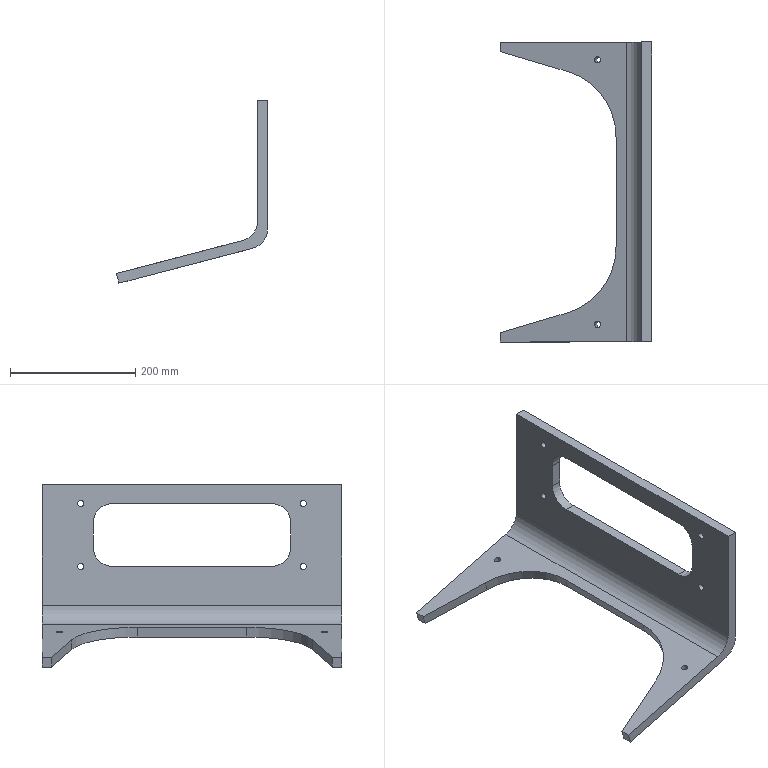Part | SolidWorks | features HoleWzd 2, ICE 2, Extrusion 1 | 1 solid | 48 faces | box 241.053 x 478 x 290.926 mm | volume 1872027 mm3 | cylinder 20 | plane 16 | cone 12 | commonest cylinder face diameters 10.2 x12 60.6 x4 64 x2 218.4 x2
STEP:
#1=CARTESIAN_POINT('',(2428.148,450.,-1751.717));
#2=VERTEX_POINT('',#1);
#3=CARTESIAN_POINT('',(2418.279,450.,-1754.295));
#4=VERTEX_POINT('',#3);
#5=CARTESIAN_POINT('',(2423.214,450.,-1753.006));
#6=DIRECTION('',(0.2527,0.,-0.9675));
#7=DIRECTION('',(-0.9675,0.,-0.2527));
#8=AXIS2_PLACEMENT_3D('',#5,#6,#7);
#9=CIRCLE('',#8,5.1);
#10=EDGE_CURVE('',#2,#4,#9,.T.);
#11=ORIENTED_EDGE('',*,*,#10,.F.);
#12=CARTESIAN_POINT('',(2429.277,450.,-1752.378));
#13=VERTEX_POINT('',#12);
#14=CARTESIAN_POINT('',(2429.277,450.,-1752.378));
#15=DIRECTION('',(0.8629,0.,-0.5054));
#16=VECTOR('',#15,1000.);
#17=LINE('',#14,#16);
#18=EDGE_CURVE('',#2,#13,#17,.T.);
#19=ORIENTED_EDGE('',*,*,#18,.T.);
#20=CARTESIAN_POINT('',(2417.618,450.,-1755.424));
#21=VERTEX_POINT('',#20);
#22=CARTESIAN_POINT('',(2423.447,450.,-1753.901));
#23=DIRECTION('',(0.2527,0.,-0.9675));
#24=DIRECTION('',(-0.9675,0.,-0.2527));
#25=AXIS2_PLACEMENT_3D('',#22,#23,#24);
#26=CIRCLE('',#25,6.025);
#27=EDGE_CURVE('',#13,#21,#26,.T.);
#28=ORIENTED_EDGE('',*,*,#27,.T.);
#29=CARTESIAN_POINT('',(2417.618,450.,-1755.424));
#30=DIRECTION('',(-0.5054,0.,-0.8629));
#31=VECTOR('',#30,1000.);
#32=LINE('',#29,#31);
#33=EDGE_CURVE('',#4,#21,#32,.T.);
#34=ORIENTED_EDGE('',*,*,#33,.F.);
#35=EDGE_LOOP('',(#11,#19,#28,#34));
#36=FACE_OUTER_BOUND('',#35,.T.);
#37=CARTESIAN_POINT('',(2423.447,450.,-1753.901));
#38=DIRECTION('',(0.2527,0.,-0.9675));
#39=DIRECTION('',(-0.9675,0.,-0.2527));
#40=AXIS2_PLACEMENT_3D('',#37,#38,#39);
#41=CONICAL_SURFACE('',#40,6.025,0.7854);
#42=ADVANCED_FACE('',(#36),#41,.F.);
#43=CARTESIAN_POINT('',(2424.338,450.,-1737.131));
#44=VERTEX_POINT('',#43);
#45=CARTESIAN_POINT('',(2414.469,450.,-1739.709));
#46=VERTEX_POINT('',#45);
#47=CARTESIAN_POINT('',(2419.403,450.,-1738.42));
#48=DIRECTION('',(0.2527,0.,-0.9675));
#49=DIRECTION('',(-0.9675,0.,-0.2527));
#50=AXIS2_PLACEMENT_3D('',#47,#48,#49);
#51=CIRCLE('',#50,5.1);
#52=EDGE_CURVE('',#44,#46,#51,.T.);
#53=ORIENTED_EDGE('',*,*,#52,.F.);
#54=CARTESIAN_POINT('',(2428.382,450.,-1752.612));
#55=DIRECTION('',(0.2527,0.,-0.9675));
#56=VECTOR('',#55,1000.);
#57=LINE('',#54,#56);
#58=EDGE_CURVE('',#44,#2,#57,.T.);
#59=ORIENTED_EDGE('',*,*,#58,.T.);
#60=ORIENTED_EDGE('',*,*,#10,.T.);
#61=CARTESIAN_POINT('',(2418.513,450.,-1755.19));
#62=DIRECTION('',(0.2527,0.,-0.9675));
#63=VECTOR('',#62,1000.);
#64=LINE('',#61,#63);
#65=EDGE_CURVE('',#46,#4,#64,.T.);
#66=ORIENTED_EDGE('',*,*,#65,.F.);
#67=EDGE_LOOP('',(#53,#59,#60,#66));
#68=FACE_OUTER_BOUND('',#67,.T.);
#69=CARTESIAN_POINT('',(2423.447,450.,-1753.901));
#70=DIRECTION('',(0.2527,0.,-0.9675));
#71=DIRECTION('',(-0.9675,0.,-0.2527));
#72=AXIS2_PLACEMENT_3D('',#69,#70,#71);
#73=CYLINDRICAL_SURFACE('',#72,5.1);
#74=ADVANCED_FACE('',(#68),#73,.F.);
#75=CARTESIAN_POINT('',(2428.148,28.,-1751.717));
#76=VERTEX_POINT('',#75);
#77=CARTESIAN_POINT('',(2418.279,28.,-1754.295));
#78=VERTEX_POINT('',#77);
#79=CARTESIAN_POINT('',(2423.214,28.,-1753.006));
#80=DIRECTION('',(0.2527,0.,-0.9675));
#81=DIRECTION('',(-0.9675,0.,-0.2527));
#82=AXIS2_PLACEMENT_3D('',#79,#80,#81);
#83=CIRCLE('',#82,5.1);
#84=EDGE_CURVE('',#76,#78,#83,.T.);
#85=ORIENTED_EDGE('',*,*,#84,.F.);
#86=CARTESIAN_POINT('',(2429.277,28.,-1752.378));
#87=VERTEX_POINT('',#86);
#88=CARTESIAN_POINT('',(2429.277,28.,-1752.378));
#89=DIRECTION('',(0.8629,0.,-0.5054));
#90=VECTOR('',#89,1000.);
#91=LINE('',#88,#90);
#92=EDGE_CURVE('',#76,#87,#91,.T.);
#93=ORIENTED_EDGE('',*,*,#92,.T.);
#94=CARTESIAN_POINT('',(2417.618,28.,-1755.424));
#95=VERTEX_POINT('',#94);
#96=CARTESIAN_POINT('',(2423.447,28.,-1753.901));
#97=DIRECTION('',(0.2527,0.,-0.9675));
#98=DIRECTION('',(-0.9675,0.,-0.2527));
#99=AXIS2_PLACEMENT_3D('',#96,#97,#98);
#100=CIRCLE('',#99,6.025);
#101=EDGE_CURVE('',#87,#95,#100,.T.);
#102=ORIENTED_EDGE('',*,*,#101,.T.);
#103=CARTESIAN_POINT('',(2417.618,28.,-1755.424));
#104=DIRECTION('',(-0.5054,0.,-0.8629));
#105=VECTOR('',#104,1000.);
#106=LINE('',#103,#105);
#107=EDGE_CURVE('',#78,#95,#106,.T.);
#108=ORIENTED_EDGE('',*,*,#107,.F.);
#109=EDGE_LOOP('',(#85,#93,#102,#108));
#110=FACE_OUTER_BOUND('',#109,.T.);
#111=CARTESIAN_POINT('',(2423.447,28.,-1753.901));
#112=DIRECTION('',(0.2527,0.,-0.9675));
#113=DIRECTION('',(-0.9675,0.,-0.2527));
#114=AXIS2_PLACEMENT_3D('',#111,#112,#113);
#115=CONICAL_SURFACE('',#114,6.025,0.7854);
#116=ADVANCED_FACE('',(#110),#115,.F.);
#117=CARTESIAN_POINT('',(2424.338,28.,-1737.131));
#118=VERTEX_POINT('',#117);
#119=CARTESIAN_POINT('',(2414.469,28.,-1739.709));
#120=VERTEX_POINT('',#119);
#121=CARTESIAN_POINT('',(2419.403,28.,-1738.42));
#122=DIRECTION('',(0.2527,0.,-0.9675));
#123=DIRECTION('',(-0.9675,0.,-0.2527));
#124=AXIS2_PLACEMENT_3D('',#121,#122,#123);
#125=CIRCLE('',#124,5.1);
#126=EDGE_CURVE('',#118,#120,#125,.T.);
#127=ORIENTED_EDGE('',*,*,#126,.F.);
#128=CARTESIAN_POINT('',(2428.382,28.,-1752.612));
#129=DIRECTION('',(0.2527,0.,-0.9675));
#130=VECTOR('',#129,1000.);
#131=LINE('',#128,#130);
#132=EDGE_CURVE('',#118,#76,#131,.T.);
#133=ORIENTED_EDGE('',*,*,#132,.T.);
#134=ORIENTED_EDGE('',*,*,#84,.T.);
#135=CARTESIAN_POINT('',(2418.513,28.,-1755.19));
#136=DIRECTION('',(0.2527,0.,-0.9675));
#137=VECTOR('',#136,1000.);
#138=LINE('',#135,#137);
#139=EDGE_CURVE('',#120,#78,#138,.T.);
#140=ORIENTED_EDGE('',*,*,#139,.F.);
#141=EDGE_LOOP('',(#127,#133,#134,#140));
#142=FACE_OUTER_BOUND('',#141,.T.);
#143=CARTESIAN_POINT('',(2423.447,28.,-1753.901));
#144=DIRECTION('',(0.2527,0.,-0.9675));
#145=DIRECTION('',(-0.9675,0.,-0.2527));
#146=AXIS2_PLACEMENT_3D('',#143,#144,#145);
#147=CYLINDRICAL_SURFACE('',#146,5.1);
#148=ADVANCED_FACE('',(#142),#147,.F.);
#149=CARTESIAN_POINT('',(2504.822,416.55,-1628.488));
#150=VERTEX_POINT('',#149);
#151=CARTESIAN_POINT('',(2504.822,416.55,-1638.688));
#152=VERTEX_POINT('',#151);
#153=CARTESIAN_POINT('',(2504.822,416.55,-1633.588));
#154=DIRECTION('',(1.,0.,0.));
#155=DIRECTION('',(0.,0.,-1.));
#156=AXIS2_PLACEMENT_3D('',#153,#154,#155);
#157=CIRCLE('',#156,5.1);
#158=EDGE_CURVE('',#150,#152,#157,.T.);
#159=ORIENTED_EDGE('',*,*,#158,.F.);
#160=CARTESIAN_POINT('',(2505.747,416.55,-1627.563));
#161=VERTEX_POINT('',#160);
#162=CARTESIAN_POINT('',(2505.747,416.55,-1627.563));
#163=DIRECTION('',(0.7071,0.,0.7071));
#164=VECTOR('',#163,1000.);
#165=LINE('',#162,#164);
#166=EDGE_CURVE('',#150,#161,#165,.T.);
#167=ORIENTED_EDGE('',*,*,#166,.T.);
#168=CARTESIAN_POINT('',(2505.747,416.55,-1639.613));
#169=VERTEX_POINT('',#168);
#170=CARTESIAN_POINT('',(2505.747,416.55,-1633.588));
#171=DIRECTION('',(1.,0.,0.));
#172=DIRECTION('',(0.,0.,-1.));
#173=AXIS2_PLACEMENT_3D('',#170,#171,#172);
#174=CIRCLE('',#173,6.025);
#175=EDGE_CURVE('',#161,#169,#174,.T.);
#176=ORIENTED_EDGE('',*,*,#175,.T.);
#177=CARTESIAN_POINT('',(2505.747,416.55,-1639.613));
#178=DIRECTION('',(0.7071,0.,-0.7071));
#179=VECTOR('',#178,1000.);
#180=LINE('',#177,#179);
#181=EDGE_CURVE('',#152,#169,#180,.T.);
#182=ORIENTED_EDGE('',*,*,#181,.F.);
#183=EDGE_LOOP('',(#159,#167,#176,#182));
#184=FACE_OUTER_BOUND('',#183,.T.);
#185=CARTESIAN_POINT('',(2505.747,416.55,-1633.588));
#186=DIRECTION('',(1.,0.,0.));
#187=DIRECTION('',(0.,0.,-1.));
#188=AXIS2_PLACEMENT_3D('',#185,#186,#187);
#189=CONICAL_SURFACE('',#188,6.025,0.7854);
#190=ADVANCED_FACE('',(#184),#189,.F.);
#191=CARTESIAN_POINT('',(2489.747,416.55,-1628.488));
#192=VERTEX_POINT('',#191);
#193=CARTESIAN_POINT('',(2489.747,416.55,-1638.688));
#194=VERTEX_POINT('',#193);
#195=CARTESIAN_POINT('',(2489.747,416.55,-1633.588));
#196=DIRECTION('',(1.,0.,0.));
#197=DIRECTION('',(0.,0.,-1.));
#198=AXIS2_PLACEMENT_3D('',#195,#196,#197);
#199=CIRCLE('',#198,5.1);
#200=EDGE_CURVE('',#192,#194,#199,.T.);
#201=ORIENTED_EDGE('',*,*,#200,.F.);
#202=CARTESIAN_POINT('',(2505.747,416.55,-1628.488));
#203=DIRECTION('',(1.,0.,0.));
#204=VECTOR('',#203,1000.);
#205=LINE('',#202,#204);
#206=EDGE_CURVE('',#192,#150,#205,.T.);
#207=ORIENTED_EDGE('',*,*,#206,.T.);
#208=ORIENTED_EDGE('',*,*,#158,.T.);
#209=CARTESIAN_POINT('',(2505.747,416.55,-1638.688));
#210=DIRECTION('',(1.,0.,0.));
#211=VECTOR('',#210,1000.);
#212=LINE('',#209,#211);
#213=EDGE_CURVE('',#194,#152,#212,.T.);
#214=ORIENTED_EDGE('',*,*,#213,.F.);
#215=EDGE_LOOP('',(#201,#207,#208,#214));
#216=FACE_OUTER_BOUND('',#215,.T.);
#217=CARTESIAN_POINT('',(2505.747,416.55,-1633.588));
#218=DIRECTION('',(1.,0.,0.));
#219=DIRECTION('',(0.,0.,-1.));
#220=AXIS2_PLACEMENT_3D('',#217,#218,#219);
#221=CYLINDRICAL_SURFACE('',#220,5.1);
#222=ADVANCED_FACE('',(#216),#221,.F.);
#223=CARTESIAN_POINT('',(2504.822,61.45,-1528.288));
#224=VERTEX_POINT('',#223);
#225=CARTESIAN_POINT('',(2504.822,61.45,-1538.488));
#226=VERTEX_POINT('',#225);
#227=CARTESIAN_POINT('',(2504.822,61.45,-1533.388));
#228=DIRECTION('',(1.,0.,0.));
#229=DIRECTION('',(0.,0.,-1.));
#230=AXIS2_PLACEMENT_3D('',#227,#228,#229);
#231=CIRCLE('',#230,5.1);
#232=EDGE_CURVE('',#224,#226,#231,.T.);
#233=ORIENTED_EDGE('',*,*,#232,.F.);
#234=CARTESIAN_POINT('',(2505.747,61.45,-1527.363));
#235=VERTEX_POINT('',#234);
#236=CARTESIAN_POINT('',(2505.747,61.45,-1527.363));
#237=DIRECTION('',(0.7071,0.,0.7071));
#238=VECTOR('',#237,1000.);
#239=LINE('',#236,#238);
#240=EDGE_CURVE('',#224,#235,#239,.T.);
#241=ORIENTED_EDGE('',*,*,#240,.T.);
#242=CARTESIAN_POINT('',(2505.747,61.45,-1539.413));
#243=VERTEX_POINT('',#242);
#244=CARTESIAN_POINT('',(2505.747,61.45,-1533.388));
#245=DIRECTION('',(1.,0.,0.));
#246=DIRECTION('',(0.,0.,-1.));
#247=AXIS2_PLACEMENT_3D('',#244,#245,#246);
#248=CIRCLE('',#247,6.025);
#249=EDGE_CURVE('',#235,#243,#248,.T.);
#250=ORIENTED_EDGE('',*,*,#249,.T.);
#251=CARTESIAN_POINT('',(2505.747,61.45,-1539.413));
#252=DIRECTION('',(0.7071,0.,-0.7071));
#253=VECTOR('',#252,1000.);
#254=LINE('',#251,#253);
#255=EDGE_CURVE('',#226,#243,#254,.T.);
#256=ORIENTED_EDGE('',*,*,#255,.F.);
#257=EDGE_LOOP('',(#233,#241,#250,#256));
#258=FACE_OUTER_BOUND('',#257,.T.);
#259=CARTESIAN_POINT('',(2505.747,61.45,-1533.388));
#260=DIRECTION('',(1.,0.,0.));
#261=DIRECTION('',(0.,0.,-1.));
#262=AXIS2_PLACEMENT_3D('',#259,#260,#261);
#263=CONICAL_SURFACE('',#262,6.025,0.7854);
#264=ADVANCED_FACE('',(#258),#263,.F.);
#265=CARTESIAN_POINT('',(2489.747,61.45,-1528.288));
#266=VERTEX_POINT('',#265);
#267=CARTESIAN_POINT('',(2489.747,61.45,-1538.488));
#268=VERTEX_POINT('',#267);
#269=CARTESIAN_POINT('',(2489.747,61.45,-1533.388));
#270=DIRECTION('',(1.,0.,0.));
#271=DIRECTION('',(0.,0.,-1.));
#272=AXIS2_PLACEMENT_3D('',#269,#270,#271);
#273=CIRCLE('',#272,5.1);
#274=EDGE_CURVE('',#266,#268,#273,.T.);
#275=ORIENTED_EDGE('',*,*,#274,.F.);
#276=CARTESIAN_POINT('',(2505.747,61.45,-1528.288));
#277=DIRECTION('',(1.,0.,0.));
#278=VECTOR('',#277,1000.);
#279=LINE('',#276,#278);
#280=EDGE_CURVE('',#266,#224,#279,.T.);
#281=ORIENTED_EDGE('',*,*,#280,.T.);
#282=ORIENTED_EDGE('',*,*,#232,.T.);
#283=CARTESIAN_POINT('',(2505.747,61.45,-1538.488));
#284=DIRECTION('',(1.,0.,0.));
#285=VECTOR('',#284,1000.);
#286=LINE('',#283,#285);
#287=EDGE_CURVE('',#268,#226,#286,.T.);
#288=ORIENTED_EDGE('',*,*,#287,.F.);
#289=EDGE_LOOP('',(#275,#281,#282,#288));
#290=FACE_OUTER_BOUND('',#289,.T.);
#291=CARTESIAN_POINT('',(2505.747,61.45,-1533.388));
#292=DIRECTION('',(1.,0.,0.));
#293=DIRECTION('',(0.,0.,-1.));
#294=AXIS2_PLACEMENT_3D('',#291,#292,#293);
#295=CYLINDRICAL_SURFACE('',#294,5.1);
#296=ADVANCED_FACE('',(#290),#295,.F.);
#297=CARTESIAN_POINT('',(2504.822,416.55,-1528.288));
#298=VERTEX_POINT('',#297);
#299=CARTESIAN_POINT('',(2504.822,416.55,-1538.488));
#300=VERTEX_POINT('',#299);
#301=CARTESIAN_POINT('',(2504.822,416.55,-1533.388));
#302=DIRECTION('',(1.,0.,0.));
#303=DIRECTION('',(0.,0.,-1.));
#304=AXIS2_PLACEMENT_3D('',#301,#302,#303);
#305=CIRCLE('',#304,5.1);
#306=EDGE_CURVE('',#298,#300,#305,.T.);
#307=ORIENTED_EDGE('',*,*,#306,.F.);
#308=CARTESIAN_POINT('',(2505.747,416.55,-1527.363));
#309=VERTEX_POINT('',#308);
#310=CARTESIAN_POINT('',(2505.747,416.55,-1527.363));
#311=DIRECTION('',(0.7071,0.,0.7071));
#312=VECTOR('',#311,1000.);
#313=LINE('',#310,#312);
#314=EDGE_CURVE('',#298,#309,#313,.T.);
#315=ORIENTED_EDGE('',*,*,#314,.T.);
#316=CARTESIAN_POINT('',(2505.747,416.55,-1539.413));
#317=VERTEX_POINT('',#316);
#318=CARTESIAN_POINT('',(2505.747,416.55,-1533.388));
#319=DIRECTION('',(1.,0.,0.));
#320=DIRECTION('',(0.,0.,-1.));
#321=AXIS2_PLACEMENT_3D('',#318,#319,#320);
#322=CIRCLE('',#321,6.025);
#323=EDGE_CURVE('',#309,#317,#322,.T.);
#324=ORIENTED_EDGE('',*,*,#323,.T.);
#325=CARTESIAN_POINT('',(2505.747,416.55,-1539.413));
#326=DIRECTION('',(0.7071,0.,-0.7071));
#327=VECTOR('',#326,1000.);
#328=LINE('',#325,#327);
#329=EDGE_CURVE('',#300,#317,#328,.T.);
#330=ORIENTED_EDGE('',*,*,#329,.F.);
#331=EDGE_LOOP('',(#307,#315,#324,#330));
#332=FACE_OUTER_BOUND('',#331,.T.);
#333=CARTESIAN_POINT('',(2505.747,416.55,-1533.388));
#334=DIRECTION('',(1.,0.,0.));
#335=DIRECTION('',(0.,0.,-1.));
#336=AXIS2_PLACEMENT_3D('',#333,#334,#335);
#337=CONICAL_SURFACE('',#336,6.025,0.7854);
#338=ADVANCED_FACE('',(#332),#337,.F.);
#339=CARTESIAN_POINT('',(2489.747,416.55,-1528.288));
#340=VERTEX_POINT('',#339);
#341=CARTESIAN_POINT('',(2489.747,416.55,-1538.488));
#342=VERTEX_POINT('',#341);
#343=CARTESIAN_POINT('',(2489.747,416.55,-1533.388));
#344=DIRECTION('',(1.,0.,0.));
#345=DIRECTION('',(0.,0.,-1.));
#346=AXIS2_PLACEMENT_3D('',#343,#344,#345);
#347=CIRCLE('',#346,5.1);
#348=EDGE_CURVE('',#340,#342,#347,.T.);
#349=ORIENTED_EDGE('',*,*,#348,.F.);
#350=CARTESIAN_POINT('',(2505.747,416.55,-1528.288));
#351=DIRECTION('',(1.,0.,0.));
#352=VECTOR('',#351,1000.);
#353=LINE('',#350,#352);
#354=EDGE_CURVE('',#340,#298,#353,.T.);
#355=ORIENTED_EDGE('',*,*,#354,.T.);
#356=ORIENTED_EDGE('',*,*,#306,.T.);
#357=CARTESIAN_POINT('',(2505.747,416.55,-1538.488));
#358=DIRECTION('',(1.,0.,0.));
#359=VECTOR('',#358,1000.);
#360=LINE('',#357,#359);
#361=EDGE_CURVE('',#342,#300,#360,.T.);
#362=ORIENTED_EDGE('',*,*,#361,.F.);
#363=EDGE_LOOP('',(#349,#355,#356,#362));
#364=FACE_OUTER_BOUND('',#363,.T.);
#365=CARTESIAN_POINT('',(2505.747,416.55,-1533.388));
#366=DIRECTION('',(1.,0.,0.));
#367=DIRECTION('',(0.,0.,-1.));
#368=AXIS2_PLACEMENT_3D('',#365,#366,#367);
#369=CYLINDRICAL_SURFACE('',#368,5.1);
#370=ADVANCED_FACE('',(#364),#369,.F.);
#371=CARTESIAN_POINT('',(2504.822,61.45,-1628.488));
#372=VERTEX_POINT('',#371);
#373=CARTESIAN_POINT('',(2504.822,61.45,-1638.688));
#374=VERTEX_POINT('',#373);
#375=CARTESIAN_POINT('',(2504.822,61.45,-1633.588));
#376=DIRECTION('',(1.,0.,0.));
#377=DIRECTION('',(0.,0.,-1.));
#378=AXIS2_PLACEMENT_3D('',#375,#376,#377);
#379=CIRCLE('',#378,5.1);
#380=EDGE_CURVE('',#372,#374,#379,.T.);
#381=ORIENTED_EDGE('',*,*,#380,.F.);
#382=CARTESIAN_POINT('',(2505.747,61.45,-1627.563));
#383=VERTEX_POINT('',#382);
#384=CARTESIAN_POINT('',(2505.747,61.45,-1627.563));
#385=DIRECTION('',(0.7071,0.,0.7071));
#386=VECTOR('',#385,1000.);
#387=LINE('',#384,#386);
#388=EDGE_CURVE('',#372,#383,#387,.T.);
#389=ORIENTED_EDGE('',*,*,#388,.T.);
#390=CARTESIAN_POINT('',(2505.747,61.45,-1639.613));
#391=VERTEX_POINT('',#390);
#392=CARTESIAN_POINT('',(2505.747,61.45,-1633.588));
#393=DIRECTION('',(1.,0.,0.));
#394=DIRECTION('',(0.,0.,-1.));
#395=AXIS2_PLACEMENT_3D('',#392,#393,#394);
#396=CIRCLE('',#395,6.025);
#397=EDGE_CURVE('',#383,#391,#396,.T.);
#398=ORIENTED_EDGE('',*,*,#397,.T.);
#399=CARTESIAN_POINT('',(2505.747,61.45,-1639.613));
#400=DIRECTION('',(0.7071,0.,-0.7071));
#401=VECTOR('',#400,1000.);
#402=LINE('',#399,#401);
#403=EDGE_CURVE('',#374,#391,#402,.T.);
#404=ORIENTED_EDGE('',*,*,#403,.F.);
#405=EDGE_LOOP('',(#381,#389,#398,#404));
#406=FACE_OUTER_BOUND('',#405,.T.);
#407=CARTESIAN_POINT('',(2505.747,61.45,-1633.588));
#408=DIRECTION('',(1.,0.,0.));
#409=DIRECTION('',(0.,0.,-1.));
#410=AXIS2_PLACEMENT_3D('',#407,#408,#409);
#411=CONICAL_SURFACE('',#410,6.025,0.7854);
#412=ADVANCED_FACE('',(#406),#411,.F.);
#413=CARTESIAN_POINT('',(2489.747,61.45,-1628.488));
#414=VERTEX_POINT('',#413);
#415=CARTESIAN_POINT('',(2489.747,61.45,-1638.688));
#416=VERTEX_POINT('',#415);
#417=CARTESIAN_POINT('',(2489.747,61.45,-1633.588));
#418=DIRECTION('',(1.,0.,0.));
#419=DIRECTION('',(0.,0.,-1.));
#420=AXIS2_PLACEMENT_3D('',#417,#418,#419);
#421=CIRCLE('',#420,5.1);
#422=EDGE_CURVE('',#414,#416,#421,.T.);
#423=ORIENTED_EDGE('',*,*,#422,.F.);
#424=CARTESIAN_POINT('',(2505.747,61.45,-1628.488));
#425=DIRECTION('',(1.,0.,0.));
#426=VECTOR('',#425,1000.);
#427=LINE('',#424,#426);
#428=EDGE_CURVE('',#414,#372,#427,.T.);
#429=ORIENTED_EDGE('',*,*,#428,.T.);
#430=ORIENTED_EDGE('',*,*,#380,.T.);
#431=CARTESIAN_POINT('',(2505.747,61.45,-1638.688));
#432=DIRECTION('',(1.,0.,0.));
#433=VECTOR('',#432,1000.);
#434=LINE('',#431,#433);
#435=EDGE_CURVE('',#416,#374,#434,.T.);
#436=ORIENTED_EDGE('',*,*,#435,.F.);
#437=EDGE_LOOP('',(#423,#429,#430,#436));
#438=FACE_OUTER_BOUND('',#437,.T.);
#439=CARTESIAN_POINT('',(2505.747,61.45,-1633.588));
#440=DIRECTION('',(1.,0.,0.));
#441=DIRECTION('',(0.,0.,-1.));
#442=AXIS2_PLACEMENT_3D('',#439,#440,#441);
#443=CYLINDRICAL_SURFACE('',#442,5.1);
#444=ADVANCED_FACE('',(#438),#443,.F.);
#445=CARTESIAN_POINT('',(2268.739,478.,-1794.315));
#446=VERTEX_POINT('',#445);
#447=CARTESIAN_POINT('',(2268.739,463.,-1794.315));
#448=VERTEX_POINT('',#447);
#449=CARTESIAN_POINT('',(2268.739,478.,-1794.315));
#450=DIRECTION('',(0.,-1.,0.));
#451=VECTOR('',#450,1000.);
#452=LINE('',#449,#451);
#453=EDGE_CURVE('',#446,#448,#452,.T.);
#454=ORIENTED_EDGE('',*,*,#453,.T.);
#455=CARTESIAN_POINT('',(2264.695,463.,-1778.834));
#456=VERTEX_POINT('',#455);
#457=CARTESIAN_POINT('',(2147.927,463.,-1331.834));
#458=DIRECTION('',(0.2527,0.,-0.9675));
#459=VECTOR('',#458,1000.);
#460=LINE('',#457,#459);
#461=EDGE_CURVE('',#456,#448,#460,.T.);
#462=ORIENTED_EDGE('',*,*,#461,.F.);
#463=CARTESIAN_POINT('',(2264.695,478.,-1778.834));
#464=VERTEX_POINT('',#463);
#465=CARTESIAN_POINT('',(2264.695,478.,-1778.834));
#466=DIRECTION('',(0.,-1.,0.));
#467=VECTOR('',#466,1000.);
#468=LINE('',#465,#467);
#469=EDGE_CURVE('',#464,#456,#468,.T.);
#470=ORIENTED_EDGE('',*,*,#469,.F.);
#471=CARTESIAN_POINT('',(2268.739,478.,-1794.315));
#472=DIRECTION('',(-0.2527,0.,0.9675));
#473=VECTOR('',#472,1000.);
#474=LINE('',#471,#473);
#475=EDGE_CURVE('',#446,#464,#474,.T.);
#476=ORIENTED_EDGE('',*,*,#475,.F.);
#477=EDGE_LOOP('',(#454,#462,#470,#476));
#478=FACE_OUTER_BOUND('',#477,.T.);
#479=CARTESIAN_POINT('',(2268.739,478.,-1794.315));
#480=DIRECTION('',(0.9675,0.,0.2527));
#481=DIRECTION('',(0.2527,0.,-0.9675));
#482=AXIS2_PLACEMENT_3D('',#479,#480,#481);
#483=PLANE('',#482);
#484=ADVANCED_FACE('',(#478),#483,.F.);
#485=CARTESIAN_POINT('',(2489.747,416.55,-1633.588));
#486=DIRECTION('',(1.,0.,0.));
#487=DIRECTION('',(0.,0.,-1.));
#488=AXIS2_PLACEMENT_3D('',#485,#486,#487);
#489=CIRCLE('',#488,5.1);
#490=EDGE_CURVE('',#194,#192,#489,.T.);
#491=ORIENTED_EDGE('',*,*,#490,.T.);
#492=ORIENTED_EDGE('',*,*,#200,.T.);
#493=EDGE_LOOP('',(#491,#492));
#494=FACE_BOUND('',#493,.T.);
#495=CARTESIAN_POINT('',(2489.747,61.45,-1533.388));
#496=DIRECTION('',(1.,0.,0.));
#497=DIRECTION('',(0.,0.,-1.));
#498=AXIS2_PLACEMENT_3D('',#495,#496,#497);
#499=CIRCLE('',#498,5.1);
#500=EDGE_CURVE('',#268,#266,#499,.T.);
#501=ORIENTED_EDGE('',*,*,#500,.T.);
#502=ORIENTED_EDGE('',*,*,#274,.T.);
#503=EDGE_LOOP('',(#501,#502));
#504=FACE_BOUND('',#503,.T.);
#505=CARTESIAN_POINT('',(2489.747,416.55,-1533.388));
#506=DIRECTION('',(1.,0.,0.));
#507=DIRECTION('',(0.,0.,-1.));
#508=AXIS2_PLACEMENT_3D('',#505,#506,#507);
#509=CIRCLE('',#508,5.1);
#510=EDGE_CURVE('',#342,#340,#509,.T.);
#511=ORIENTED_EDGE('',*,*,#510,.T.);
#512=ORIENTED_EDGE('',*,*,#348,.T.);
#513=EDGE_LOOP('',(#511,#512));
#514=FACE_BOUND('',#513,.T.);
#515=CARTESIAN_POINT('',(2489.747,61.45,-1633.588));
#516=DIRECTION('',(1.,0.,0.));
#517=DIRECTION('',(0.,0.,-1.));
#518=AXIS2_PLACEMENT_3D('',#515,#516,#517);
#519=CIRCLE('',#518,5.1);
#520=EDGE_CURVE('',#416,#414,#519,.T.);
#521=ORIENTED_EDGE('',*,*,#520,.T.);
#522=ORIENTED_EDGE('',*,*,#422,.T.);
#523=EDGE_LOOP('',(#521,#522));
#524=FACE_BOUND('',#523,.T.);
#525=CARTESIAN_POINT('',(2489.747,366.1,-1533.388));
#526=VERTEX_POINT('',#525);
#527=CARTESIAN_POINT('',(2489.747,111.9,-1533.388));
#528=VERTEX_POINT('',#527);
#529=CARTESIAN_POINT('',(2489.747,478.,-1533.388));
#530=DIRECTION('',(0.,-1.,0.));
#531=VECTOR('',#530,1000.);
#532=LINE('',#529,#531);
#533=EDGE_CURVE('',#526,#528,#532,.T.);
#534=ORIENTED_EDGE('',*,*,#533,.T.);
#535=CARTESIAN_POINT('',(2489.747,81.6,-1563.688));
#536=VERTEX_POINT('',#535);
#537=CARTESIAN_POINT('',(2489.747,111.9,-1563.688));
#538=DIRECTION('',(1.,0.,0.));
#539=DIRECTION('',(0.,0.,-1.));
#540=AXIS2_PLACEMENT_3D('',#537,#538,#539);
#541=CIRCLE('',#540,30.3);
#542=EDGE_CURVE('',#528,#536,#541,.T.);
#543=ORIENTED_EDGE('',*,*,#542,.T.);
#544=CARTESIAN_POINT('',(2489.747,81.6,-1603.288));
#545=VERTEX_POINT('',#544);
#546=CARTESIAN_POINT('',(2489.747,81.6,-1503.388));
#547=DIRECTION('',(0.,0.,-1.));
#548=VECTOR('',#547,1000.);
#549=LINE('',#546,#548);
#550=EDGE_CURVE('',#536,#545,#549,.T.);
#551=ORIENTED_EDGE('',*,*,#550,.T.);
#552=CARTESIAN_POINT('',(2489.747,111.9,-1633.588));
#553=VERTEX_POINT('',#552);
#554=CARTESIAN_POINT('',(2489.747,111.9,-1603.288));
#555=DIRECTION('',(1.,0.,0.));
#556=DIRECTION('',(0.,0.,-1.));
#557=AXIS2_PLACEMENT_3D('',#554,#555,#556);
#558=CIRCLE('',#557,30.3);
#559=EDGE_CURVE('',#545,#553,#558,.T.);
#560=ORIENTED_EDGE('',*,*,#559,.T.);
#561=CARTESIAN_POINT('',(2489.747,366.1,-1633.588));
#562=VERTEX_POINT('',#561);
#563=CARTESIAN_POINT('',(2489.747,478.,-1633.588));
#564=DIRECTION('',(0.,1.,0.));
#565=VECTOR('',#564,1000.);
#566=LINE('',#563,#565);
#567=EDGE_CURVE('',#553,#562,#566,.T.);
#568=ORIENTED_EDGE('',*,*,#567,.T.);
#569=CARTESIAN_POINT('',(2489.747,396.4,-1603.288));
#570=VERTEX_POINT('',#569);
#571=CARTESIAN_POINT('',(2489.747,366.1,-1603.288));
#572=DIRECTION('',(1.,0.,0.));
#573=DIRECTION('',(0.,0.,-1.));
#574=AXIS2_PLACEMENT_3D('',#571,#572,#573);
#575=CIRCLE('',#574,30.3);
#576=EDGE_CURVE('',#562,#570,#575,.T.);
#577=ORIENTED_EDGE('',*,*,#576,.T.);
#578=CARTESIAN_POINT('',(2489.747,396.4,-1563.688));
#579=VERTEX_POINT('',#578);
#580=CARTESIAN_POINT('',(2489.747,396.4,-1503.388));
#581=DIRECTION('',(0.,0.,1.));
#582=VECTOR('',#581,1000.);
#583=LINE('',#580,#582);
#584=EDGE_CURVE('',#570,#579,#583,.T.);
#585=ORIENTED_EDGE('',*,*,#584,.T.);
#586=CARTESIAN_POINT('',(2489.747,366.1,-1563.688));
#587=DIRECTION('',(1.,0.,0.));
#588=DIRECTION('',(0.,0.,-1.));
#589=AXIS2_PLACEMENT_3D('',#586,#587,#588);
#590=CIRCLE('',#589,30.3);
#591=EDGE_CURVE('',#579,#526,#590,.T.);
#592=ORIENTED_EDGE('',*,*,#591,.T.);
#593=EDGE_LOOP('',(#534,#543,#551,#560,#568,#577,#585,#592));
#594=FACE_BOUND('',#593,.T.);
#595=CARTESIAN_POINT('',(2489.747,0.,-1695.33));
#596=VERTEX_POINT('',#595);
#597=CARTESIAN_POINT('',(2489.747,0.,-1503.388));
#598=VERTEX_POINT('',#597);
#599=CARTESIAN_POINT('',(2489.747,0.,-1503.388));
#600=DIRECTION('',(0.,0.,1.));
#601=VECTOR('',#600,1000.);
#602=LINE('',#599,#601);
#603=EDGE_CURVE('',#596,#598,#602,.T.);
#604=ORIENTED_EDGE('',*,*,#603,.T.);
#605=CARTESIAN_POINT('',(2489.747,478.,-1503.388));
#606=VERTEX_POINT('',#605);
#607=CARTESIAN_POINT('',(2489.747,478.,-1503.388));
#608=DIRECTION('',(0.,-1.,0.));
#609=VECTOR('',#608,1000.);
#610=LINE('',#607,#609);
#611=EDGE_CURVE('',#606,#598,#610,.T.);
#612=ORIENTED_EDGE('',*,*,#611,.F.);
#613=CARTESIAN_POINT('',(2489.747,478.,-1695.33));
#614=VERTEX_POINT('',#613);
#615=CARTESIAN_POINT('',(2489.747,478.,-1503.388));
#616=DIRECTION('',(0.,0.,1.));
#617=VECTOR('',#616,1000.);
#618=LINE('',#615,#617);
#619=EDGE_CURVE('',#614,#606,#618,.T.);
#620=ORIENTED_EDGE('',*,*,#619,.F.);
#621=CARTESIAN_POINT('',(2489.747,478.,-1695.33));
#622=DIRECTION('',(0.,-1.,0.));
#623=VECTOR('',#622,1000.);
#624=LINE('',#621,#623);
#625=EDGE_CURVE('',#614,#596,#624,.T.);
#626=ORIENTED_EDGE('',*,*,#625,.T.);
#627=EDGE_LOOP('',(#604,#612,#620,#626));
#628=FACE_OUTER_BOUND('',#627,.T.);
#629=CARTESIAN_POINT('',(2489.747,478.,-1503.388));
#630=DIRECTION('',(1.,0.,0.));
#631=DIRECTION('',(0.,0.,-1.));
#632=AXIS2_PLACEMENT_3D('',#629,#630,#631);
#633=PLANE('',#632);
#634=ADVANCED_FACE('',(#494,#504,#514,#524,#594,#628),#633,.F.);
#635=CARTESIAN_POINT('',(2505.747,0.,-1503.388));
#636=VERTEX_POINT('',#635);
#637=CARTESIAN_POINT('',(2489.747,0.,-1503.388));
#638=DIRECTION('',(1.,0.,0.));
#639=VECTOR('',#638,1000.);
#640=LINE('',#637,#639);
#641=EDGE_CURVE('',#598,#636,#640,.T.);
#642=ORIENTED_EDGE('',*,*,#641,.T.);
#643=CARTESIAN_POINT('',(2505.747,478.,-1503.388));
#644=VERTEX_POINT('',#643);
#645=CARTESIAN_POINT('',(2505.747,478.,-1503.388));
#646=DIRECTION('',(0.,-1.,0.));
#647=VECTOR('',#646,1000.);
#648=LINE('',#645,#647);
#649=EDGE_CURVE('',#644,#636,#648,.T.);
#650=ORIENTED_EDGE('',*,*,#649,.F.);
#651=CARTESIAN_POINT('',(2489.747,478.,-1503.388));
#652=DIRECTION('',(1.,0.,0.));
#653=VECTOR('',#652,1000.);
#654=LINE('',#651,#653);
#655=EDGE_CURVE('',#606,#644,#654,.T.);
#656=ORIENTED_EDGE('',*,*,#655,.F.);
#657=ORIENTED_EDGE('',*,*,#611,.T.);
#658=EDGE_LOOP('',(#642,#650,#656,#657));
#659=FACE_OUTER_BOUND('',#658,.T.);
#660=CARTESIAN_POINT('',(2489.747,478.,-1503.388));
#661=DIRECTION('',(0.,0.,-1.));
#662=DIRECTION('',(-1.,0.,0.));
#663=AXIS2_PLACEMENT_3D('',#660,#661,#662);
#664=PLANE('',#663);
#665=ADVANCED_FACE('',(#659),#664,.F.);
#666=CARTESIAN_POINT('',(2505.747,416.55,-1633.588));
#667=DIRECTION('',(1.,0.,0.));
#668=DIRECTION('',(0.,0.,-1.));
#669=AXIS2_PLACEMENT_3D('',#666,#667,#668);
#670=CIRCLE('',#669,6.025);
#671=EDGE_CURVE('',#169,#161,#670,.T.);
#672=ORIENTED_EDGE('',*,*,#671,.F.);
#673=ORIENTED_EDGE('',*,*,#175,.F.);
#674=EDGE_LOOP('',(#672,#673));
#675=FACE_BOUND('',#674,.T.);
#676=CARTESIAN_POINT('',(2505.747,61.45,-1533.388));
#677=DIRECTION('',(1.,0.,0.));
#678=DIRECTION('',(0.,0.,-1.));
#679=AXIS2_PLACEMENT_3D('',#676,#677,#678);
#680=CIRCLE('',#679,6.025);
#681=EDGE_CURVE('',#243,#235,#680,.T.);
#682=ORIENTED_EDGE('',*,*,#681,.F.);
#683=ORIENTED_EDGE('',*,*,#249,.F.);
#684=EDGE_LOOP('',(#682,#683));
#685=FACE_BOUND('',#684,.T.);
#686=CARTESIAN_POINT('',(2505.747,416.55,-1533.388));
#687=DIRECTION('',(1.,0.,0.));
#688=DIRECTION('',(0.,0.,-1.));
#689=AXIS2_PLACEMENT_3D('',#686,#687,#688);
#690=CIRCLE('',#689,6.025);
#691=EDGE_CURVE('',#317,#309,#690,.T.);
#692=ORIENTED_EDGE('',*,*,#691,.F.);
#693=ORIENTED_EDGE('',*,*,#323,.F.);
#694=EDGE_LOOP('',(#692,#693));
#695=FACE_BOUND('',#694,.T.);
#696=CARTESIAN_POINT('',(2505.747,61.45,-1633.588));
#697=DIRECTION('',(1.,0.,0.));
#698=DIRECTION('',(0.,0.,-1.));
#699=AXIS2_PLACEMENT_3D('',#696,#697,#698);
#700=CIRCLE('',#699,6.025);
#701=EDGE_CURVE('',#391,#383,#700,.T.);
#702=ORIENTED_EDGE('',*,*,#701,.F.);
#703=ORIENTED_EDGE('',*,*,#397,.F.);
#704=EDGE_LOOP('',(#702,#703));
#705=FACE_BOUND('',#704,.T.);
#706=CARTESIAN_POINT('',(2505.747,81.6,-1563.688));
#707=VERTEX_POINT('',#706);
#708=CARTESIAN_POINT('',(2505.747,81.6,-1603.288));
#709=VERTEX_POINT('',#708);
#710=CARTESIAN_POINT('',(2505.747,81.6,-1563.688));
#711=DIRECTION('',(0.,0.,-1.));
#712=VECTOR('',#711,1000.);
#713=LINE('',#710,#712);
#714=EDGE_CURVE('',#707,#709,#713,.T.);
#715=ORIENTED_EDGE('',*,*,#714,.F.);
#716=CARTESIAN_POINT('',(2505.747,111.9,-1533.388));
#717=VERTEX_POINT('',#716);
#718=CARTESIAN_POINT('',(2505.747,111.9,-1563.688));
#719=DIRECTION('',(1.,0.,0.));
#720=DIRECTION('',(0.,0.,1.));
#721=AXIS2_PLACEMENT_3D('',#718,#719,#720);
#722=CIRCLE('',#721,30.3);
#723=EDGE_CURVE('',#717,#707,#722,.T.);
#724=ORIENTED_EDGE('',*,*,#723,.F.);
#725=CARTESIAN_POINT('',(2505.747,366.1,-1533.388));
#726=VERTEX_POINT('',#725);
#727=CARTESIAN_POINT('',(2505.747,111.9,-1533.388));
#728=DIRECTION('',(0.,-1.,0.));
#729=VECTOR('',#728,1000.);
#730=LINE('',#727,#729);
#731=EDGE_CURVE('',#726,#717,#730,.T.);
#732=ORIENTED_EDGE('',*,*,#731,.F.);
#733=CARTESIAN_POINT('',(2505.747,396.4,-1563.688));
#734=VERTEX_POINT('',#733);
#735=CARTESIAN_POINT('',(2505.747,366.1,-1563.688));
#736=DIRECTION('',(1.,0.,0.));
#737=DIRECTION('',(0.,0.,1.));
#738=AXIS2_PLACEMENT_3D('',#735,#736,#737);
#739=CIRCLE('',#738,30.3);
#740=EDGE_CURVE('',#734,#726,#739,.T.);
#741=ORIENTED_EDGE('',*,*,#740,.F.);
#742=CARTESIAN_POINT('',(2505.747,396.4,-1603.288));
#743=VERTEX_POINT('',#742);
#744=CARTESIAN_POINT('',(2505.747,396.4,-1563.688));
#745=DIRECTION('',(0.,0.,1.));
#746=VECTOR('',#745,1000.);
#747=LINE('',#744,#746);
#748=EDGE_CURVE('',#743,#734,#747,.T.);
#749=ORIENTED_EDGE('',*,*,#748,.F.);
#750=CARTESIAN_POINT('',(2505.747,366.1,-1633.588));
#751=VERTEX_POINT('',#750);
#752=CARTESIAN_POINT('',(2505.747,366.1,-1603.288));
#753=DIRECTION('',(1.,0.,0.));
#754=DIRECTION('',(0.,0.,1.));
#755=AXIS2_PLACEMENT_3D('',#752,#753,#754);
#756=CIRCLE('',#755,30.3);
#757=EDGE_CURVE('',#751,#743,#756,.T.);
#758=ORIENTED_EDGE('',*,*,#757,.F.);
#759=CARTESIAN_POINT('',(2505.747,111.9,-1633.588));
#760=VERTEX_POINT('',#759);
#761=CARTESIAN_POINT('',(2505.747,111.9,-1633.588));
#762=DIRECTION('',(0.,1.,0.));
#763=VECTOR('',#762,1000.);
#764=LINE('',#761,#763);
#765=EDGE_CURVE('',#760,#751,#764,.T.);
#766=ORIENTED_EDGE('',*,*,#765,.F.);
#767=CARTESIAN_POINT('',(2505.747,111.9,-1603.288));
#768=DIRECTION('',(1.,0.,0.));
#769=DIRECTION('',(0.,0.,-1.));
#770=AXIS2_PLACEMENT_3D('',#767,#768,#769);
#771=CIRCLE('',#770,30.3);
#772=EDGE_CURVE('',#709,#760,#771,.T.);
#773=ORIENTED_EDGE('',*,*,#772,.F.);
#774=EDGE_LOOP('',(#715,#724,#732,#741,#749,#758,#766,#773));
#775=FACE_BOUND('',#774,.T.);
#776=CARTESIAN_POINT('',(2505.747,0.,-1707.688));
#777=VERTEX_POINT('',#776);
#778=CARTESIAN_POINT('',(2505.747,0.,-1707.688));
#779=DIRECTION('',(0.,0.,-1.));
#780=VECTOR('',#779,1000.);
#781=LINE('',#778,#780);
#782=EDGE_CURVE('',#636,#777,#781,.T.);
#783=ORIENTED_EDGE('',*,*,#782,.T.);
#784=CARTESIAN_POINT('',(2505.747,478.,-1707.688));
#785=VERTEX_POINT('',#784);
#786=CARTESIAN_POINT('',(2505.747,478.,-1707.688));
#787=DIRECTION('',(0.,-1.,0.));
#788=VECTOR('',#787,1000.);
#789=LINE('',#786,#788);
#790=EDGE_CURVE('',#785,#777,#789,.T.);
#791=ORIENTED_EDGE('',*,*,#790,.F.);
#792=CARTESIAN_POINT('',(2505.747,478.,-1707.688));
#793=DIRECTION('',(0.,0.,-1.));
#794=VECTOR('',#793,1000.);
#795=LINE('',#792,#794);
#796=EDGE_CURVE('',#644,#785,#795,.T.);
#797=ORIENTED_EDGE('',*,*,#796,.F.);
#798=ORIENTED_EDGE('',*,*,#649,.T.);
#799=EDGE_LOOP('',(#783,#791,#797,#798));
#800=FACE_OUTER_BOUND('',#799,.T.);
#801=CARTESIAN_POINT('',(2505.747,478.,-1707.688));
#802=DIRECTION('',(-1.,0.,0.));
#803=DIRECTION('',(0.,0.,1.));
#804=AXIS2_PLACEMENT_3D('',#801,#802,#803);
#805=PLANE('',#804);
#806=ADVANCED_FACE('',(#675,#685,#695,#705,#775,#800),#805,.F.);
#807=CARTESIAN_POINT('',(2481.835,0.,-1738.649));
#808=VERTEX_POINT('',#807);
#809=CARTESIAN_POINT('',(2473.747,0.,-1707.688));
#810=DIRECTION('',(0.,1.,0.));
#811=DIRECTION('',(0.,0.,1.));
#812=AXIS2_PLACEMENT_3D('',#809,#810,#811);
#813=CIRCLE('',#812,32.);
#814=EDGE_CURVE('',#777,#808,#813,.T.);
#815=ORIENTED_EDGE('',*,*,#814,.T.);
#816=CARTESIAN_POINT('',(2481.835,478.,-1738.649));
#817=VERTEX_POINT('',#816);
#818=CARTESIAN_POINT('',(2481.835,478.,-1738.649));
#819=DIRECTION('',(0.,-1.,0.));
#820=VECTOR('',#819,1000.);
#821=LINE('',#818,#820);
#822=EDGE_CURVE('',#817,#808,#821,.T.);
#823=ORIENTED_EDGE('',*,*,#822,.F.);
#824=CARTESIAN_POINT('',(2473.747,478.,-1707.688));
#825=DIRECTION('',(0.,1.,0.));
#826=DIRECTION('',(0.,0.,1.));
#827=AXIS2_PLACEMENT_3D('',#824,#825,#826);
#828=CIRCLE('',#827,32.);
#829=EDGE_CURVE('',#785,#817,#828,.T.);
#830=ORIENTED_EDGE('',*,*,#829,.F.);
#831=ORIENTED_EDGE('',*,*,#790,.T.);
#832=EDGE_LOOP('',(#815,#823,#830,#831));
#833=FACE_OUTER_BOUND('',#832,.T.);
#834=CARTESIAN_POINT('',(2473.747,478.,-1707.688));
#835=DIRECTION('',(0.,-1.,0.));
#836=DIRECTION('',(0.,0.,-1.));
#837=AXIS2_PLACEMENT_3D('',#834,#835,#836);
#838=CYLINDRICAL_SURFACE('',#837,32.);
#839=ADVANCED_FACE('',(#833),#838,.T.);
#840=CARTESIAN_POINT('',(2423.447,450.,-1753.901));
#841=DIRECTION('',(0.2527,0.,-0.9675));
#842=DIRECTION('',(-0.9675,0.,-0.2527));
#843=AXIS2_PLACEMENT_3D('',#840,#841,#842);
#844=CIRCLE('',#843,6.025);
#845=EDGE_CURVE('',#21,#13,#844,.T.);
#846=ORIENTED_EDGE('',*,*,#845,.F.);
#847=ORIENTED_EDGE('',*,*,#27,.F.);
#848=EDGE_LOOP('',(#846,#847));
#849=FACE_BOUND('',#848,.T.);
#850=CARTESIAN_POINT('',(2423.447,28.,-1753.901));
#851=DIRECTION('',(0.2527,0.,-0.9675));
#852=DIRECTION('',(-0.9675,0.,-0.2527));
#853=AXIS2_PLACEMENT_3D('',#850,#851,#852);
#854=CIRCLE('',#853,6.025);
#855=EDGE_CURVE('',#95,#87,#854,.T.);
#856=ORIENTED_EDGE('',*,*,#855,.F.);
#857=ORIENTED_EDGE('',*,*,#101,.F.);
#858=EDGE_LOOP('',(#856,#857));
#859=FACE_BOUND('',#858,.T.);
#860=CARTESIAN_POINT('',(2376.618,431.028,-1766.134));
#861=VERTEX_POINT('',#860);
#862=CARTESIAN_POINT('',(2453.151,326.058,-1746.142));
#863=VERTEX_POINT('',#862);
#864=CARTESIAN_POINT('',(2347.496,326.058,-1773.741));
#865=DIRECTION('',(0.2527,0.,-0.9675));
#866=DIRECTION('',(0.9675,0.,0.2527));
#867=AXIS2_PLACEMENT_3D('',#864,#865,#866);
#868=CIRCLE('',#867,109.2);
#869=EDGE_CURVE('',#861,#863,#868,.T.);
#870=ORIENTED_EDGE('',*,*,#869,.F.);
#871=CARTESIAN_POINT('',(2376.618,431.028,-1766.134));
#872=DIRECTION('',(0.9301,-0.2756,0.243));
#873=VECTOR('',#872,1000.);
#874=LINE('',#871,#873);
#875=EDGE_CURVE('',#448,#861,#874,.T.);
#876=ORIENTED_EDGE('',*,*,#875,.F.);
#877=ORIENTED_EDGE('',*,*,#453,.F.);
#878=CARTESIAN_POINT('',(2481.835,478.,-1738.649));
#879=DIRECTION('',(-0.9675,0.,-0.2527));
#880=VECTOR('',#879,1000.);
#881=LINE('',#878,#880);
#882=EDGE_CURVE('',#817,#446,#881,.T.);
#883=ORIENTED_EDGE('',*,*,#882,.F.);
#884=ORIENTED_EDGE('',*,*,#822,.T.);
#885=CARTESIAN_POINT('',(2268.739,0.,-1794.315));
#886=VERTEX_POINT('',#885);
#887=CARTESIAN_POINT('',(2481.835,0.,-1738.649));
#888=DIRECTION('',(-0.9675,0.,-0.2527));
#889=VECTOR('',#888,1000.);
#890=LINE('',#887,#889);
#891=EDGE_CURVE('',#808,#886,#890,.T.);
#892=ORIENTED_EDGE('',*,*,#891,.T.);
#893=CARTESIAN_POINT('',(2268.739,15.,-1794.315));
#894=VERTEX_POINT('',#893);
#895=CARTESIAN_POINT('',(2268.739,478.,-1794.315));
#896=DIRECTION('',(0.,-1.,0.));
#897=VECTOR('',#896,1000.);
#898=LINE('',#895,#897);
#899=EDGE_CURVE('',#894,#886,#898,.T.);
#900=ORIENTED_EDGE('',*,*,#899,.F.);
#901=CARTESIAN_POINT('',(2376.618,46.972,-1766.134));
#902=VERTEX_POINT('',#901);
#903=CARTESIAN_POINT('',(2268.739,15.,-1794.315));
#904=DIRECTION('',(-0.9301,-0.2756,-0.243));
#905=VECTOR('',#904,1000.);
#906=LINE('',#903,#905);
#907=EDGE_CURVE('',#902,#894,#906,.T.);
#908=ORIENTED_EDGE('',*,*,#907,.F.);
#909=CARTESIAN_POINT('',(2453.151,151.942,-1746.142));
#910=VERTEX_POINT('',#909);
#911=CARTESIAN_POINT('',(2347.496,151.942,-1773.741));
#912=DIRECTION('',(0.2527,0.,-0.9675));
#913=DIRECTION('',(0.9675,0.,0.2527));
#914=AXIS2_PLACEMENT_3D('',#911,#912,#913);
#915=CIRCLE('',#914,109.2);
#916=EDGE_CURVE('',#910,#902,#915,.T.);
#917=ORIENTED_EDGE('',*,*,#916,.F.);
#918=CARTESIAN_POINT('',(2453.151,151.942,-1746.142));
#919=DIRECTION('',(0.,-1.,0.));
#920=VECTOR('',#919,1000.);
#921=LINE('',#918,#920);
#922=EDGE_CURVE('',#863,#910,#921,.T.);
#923=ORIENTED_EDGE('',*,*,#922,.F.);
#924=EDGE_LOOP('',(#870,#876,#877,#883,#884,#892,#900,#908,#917,#923));
#925=FACE_OUTER_BOUND('',#924,.T.);
#926=CARTESIAN_POINT('',(2481.835,478.,-1738.649));
#927=DIRECTION('',(-0.2527,0.,0.9675));
#928=DIRECTION('',(0.9675,0.,0.2527));
#929=AXIS2_PLACEMENT_3D('',#926,#927,#928);
#930=PLANE('',#929);
#931=ADVANCED_FACE('',(#849,#859,#925),#930,.F.);
#932=CARTESIAN_POINT('',(2264.695,15.,-1778.834));
#933=VERTEX_POINT('',#932);
#934=CARTESIAN_POINT('',(2264.695,0.,-1778.834));
#935=VERTEX_POINT('',#934);
#936=CARTESIAN_POINT('',(2264.695,478.,-1778.834));
#937=DIRECTION('',(0.,-1.,0.));
#938=VECTOR('',#937,1000.);
#939=LINE('',#936,#938);
#940=EDGE_CURVE('',#933,#935,#939,.T.);
#941=ORIENTED_EDGE('',*,*,#940,.F.);
#942=CARTESIAN_POINT('',(2147.927,15.,-1331.834));
#943=DIRECTION('',(0.2527,0.,-0.9675));
#944=VECTOR('',#943,1000.);
#945=LINE('',#942,#944);
#946=EDGE_CURVE('',#933,#894,#945,.T.);
#947=ORIENTED_EDGE('',*,*,#946,.T.);
#948=ORIENTED_EDGE('',*,*,#899,.T.);
#949=CARTESIAN_POINT('',(2268.739,0.,-1794.315));
#950=DIRECTION('',(-0.2527,0.,0.9675));
#951=VECTOR('',#950,1000.);
#952=LINE('',#949,#951);
#953=EDGE_CURVE('',#886,#935,#952,.T.);
#954=ORIENTED_EDGE('',*,*,#953,.T.);
#955=EDGE_LOOP('',(#941,#947,#948,#954));
#956=FACE_OUTER_BOUND('',#955,.T.);
#957=CARTESIAN_POINT('',(2268.739,478.,-1794.315));
#958=DIRECTION('',(0.9675,0.,0.2527));
#959=DIRECTION('',(0.2527,0.,-0.9675));
#960=AXIS2_PLACEMENT_3D('',#957,#958,#959);
#961=PLANE('',#960);
#962=ADVANCED_FACE('',(#956),#961,.F.);
#963=CARTESIAN_POINT('',(2419.403,450.,-1738.42));
#964=DIRECTION('',(0.2527,0.,-0.9675));
#965=DIRECTION('',(-0.9675,0.,-0.2527));
#966=AXIS2_PLACEMENT_3D('',#963,#964,#965);
#967=CIRCLE('',#966,5.1);
#968=EDGE_CURVE('',#46,#44,#967,.T.);
#969=ORIENTED_EDGE('',*,*,#968,.T.);
#970=ORIENTED_EDGE('',*,*,#52,.T.);
#971=EDGE_LOOP('',(#969,#970));
#972=FACE_BOUND('',#971,.T.);
#973=CARTESIAN_POINT('',(2419.403,28.,-1738.42));
#974=DIRECTION('',(0.2527,0.,-0.9675));
#975=DIRECTION('',(-0.9675,0.,-0.2527));
#976=AXIS2_PLACEMENT_3D('',#973,#974,#975);
#977=CIRCLE('',#976,5.1);
#978=EDGE_CURVE('',#120,#118,#977,.T.);
#979=ORIENTED_EDGE('',*,*,#978,.T.);
#980=ORIENTED_EDGE('',*,*,#126,.T.);
#981=EDGE_LOOP('',(#979,#980));
#982=FACE_BOUND('',#981,.T.);
#983=ORIENTED_EDGE('',*,*,#469,.T.);
#984=CARTESIAN_POINT('',(2372.574,431.028,-1750.653));
#985=VERTEX_POINT('',#984);
#986=CARTESIAN_POINT('',(2446.708,409.057,-1731.288));
#987=DIRECTION('',(0.9301,-0.2756,0.243));
#988=VECTOR('',#987,1000.);
#989=LINE('',#986,#988);
#990=EDGE_CURVE('',#456,#985,#989,.T.);
#991=ORIENTED_EDGE('',*,*,#990,.T.);
#992=CARTESIAN_POINT('',(2449.107,326.058,-1730.661));
#993=VERTEX_POINT('',#992);
#994=CARTESIAN_POINT('',(2343.452,326.058,-1758.261));
#995=DIRECTION('',(0.2527,0.,-0.9675));
#996=DIRECTION('',(-0.9675,0.,-0.2527));
#997=AXIS2_PLACEMENT_3D('',#994,#995,#996);
#998=CIRCLE('',#997,109.2);
#999=EDGE_CURVE('',#985,#993,#998,.T.);
#1000=ORIENTED_EDGE('',*,*,#999,.T.);
#1001=CARTESIAN_POINT('',(2449.107,151.942,-1730.661));
#1002=VERTEX_POINT('',#1001);
#1003=CARTESIAN_POINT('',(2449.107,478.,-1730.661));
#1004=DIRECTION('',(0.,-1.,0.));
#1005=VECTOR('',#1004,1000.);
#1006=LINE('',#1003,#1005);
#1007=EDGE_CURVE('',#993,#1002,#1006,.T.);
#1008=ORIENTED_EDGE('',*,*,#1007,.T.);
#1009=CARTESIAN_POINT('',(2372.574,46.972,-1750.653));
#1010=VERTEX_POINT('',#1009);
#1011=CARTESIAN_POINT('',(2343.452,151.942,-1758.261));
#1012=DIRECTION('',(0.2527,0.,-0.9675));
#1013=DIRECTION('',(-0.9675,0.,-0.2527));
#1014=AXIS2_PLACEMENT_3D('',#1011,#1012,#1013);
#1015=CIRCLE('',#1014,109.2);
#1016=EDGE_CURVE('',#1002,#1010,#1015,.T.);
#1017=ORIENTED_EDGE('',*,*,#1016,.T.);
#1018=CARTESIAN_POINT('',(2569.247,105.259,-1699.278));
#1019=DIRECTION('',(-0.9301,-0.2756,-0.243));
#1020=VECTOR('',#1019,1000.);
#1021=LINE('',#1018,#1020);
#1022=EDGE_CURVE('',#1010,#933,#1021,.T.);
#1023=ORIENTED_EDGE('',*,*,#1022,.T.);
#1024=ORIENTED_EDGE('',*,*,#940,.T.);
#1025=CARTESIAN_POINT('',(2465.835,0.,-1726.291));
#1026=VERTEX_POINT('',#1025);
#1027=CARTESIAN_POINT('',(2465.835,0.,-1726.291));
#1028=DIRECTION('',(0.9675,0.,0.2527));
#1029=VECTOR('',#1028,1000.);
#1030=LINE('',#1027,#1029);
#1031=EDGE_CURVE('',#935,#1026,#1030,.T.);
#1032=ORIENTED_EDGE('',*,*,#1031,.T.);
#1033=CARTESIAN_POINT('',(2465.835,478.,-1726.291));
#1034=VERTEX_POINT('',#1033);
#1035=CARTESIAN_POINT('',(2465.835,478.,-1726.291));
#1036=DIRECTION('',(0.,-1.,0.));
#1037=VECTOR('',#1036,1000.);
#1038=LINE('',#1035,#1037);
#1039=EDGE_CURVE('',#1034,#1026,#1038,.T.);
#1040=ORIENTED_EDGE('',*,*,#1039,.F.);
#1041=CARTESIAN_POINT('',(2465.835,478.,-1726.291));
#1042=DIRECTION('',(0.9675,0.,0.2527));
#1043=VECTOR('',#1042,1000.);
#1044=LINE('',#1041,#1043);
#1045=EDGE_CURVE('',#464,#1034,#1044,.T.);
#1046=ORIENTED_EDGE('',*,*,#1045,.F.);
#1047=EDGE_LOOP('',(#983,#991,#1000,#1008,#1017,#1023,#1024,#1032,#1040,#1046));
#1048=FACE_OUTER_BOUND('',#1047,.T.);
#1049=CARTESIAN_POINT('',(2465.835,478.,-1726.291));
#1050=DIRECTION('',(0.2527,0.,-0.9675));
#1051=DIRECTION('',(-0.9675,0.,-0.2527));
#1052=AXIS2_PLACEMENT_3D('',#1049,#1050,#1051);
#1053=PLANE('',#1052);
#1054=ADVANCED_FACE('',(#972,#982,#1048),#1053,.F.);
#1055=CARTESIAN_POINT('',(2457.747,0.,-1695.33));
#1056=DIRECTION('',(0.,-1.,0.));
#1057=DIRECTION('',(0.,0.,1.));
#1058=AXIS2_PLACEMENT_3D('',#1055,#1056,#1057);
#1059=CIRCLE('',#1058,32.);
#1060=EDGE_CURVE('',#1026,#596,#1059,.T.);
#1061=ORIENTED_EDGE('',*,*,#1060,.T.);
#1062=ORIENTED_EDGE('',*,*,#625,.F.);
#1063=CARTESIAN_POINT('',(2457.747,478.,-1695.33));
#1064=DIRECTION('',(0.,-1.,0.));
#1065=DIRECTION('',(0.,0.,1.));
#1066=AXIS2_PLACEMENT_3D('',#1063,#1064,#1065);
#1067=CIRCLE('',#1066,32.);
#1068=EDGE_CURVE('',#1034,#614,#1067,.T.);
#1069=ORIENTED_EDGE('',*,*,#1068,.F.);
#1070=ORIENTED_EDGE('',*,*,#1039,.T.);
#1071=EDGE_LOOP('',(#1061,#1062,#1069,#1070));
#1072=FACE_OUTER_BOUND('',#1071,.T.);
#1073=CARTESIAN_POINT('',(2457.747,478.,-1695.33));
#1074=DIRECTION('',(0.,-1.,0.));
#1075=DIRECTION('',(0.,0.,-1.));
#1076=AXIS2_PLACEMENT_3D('',#1073,#1074,#1075);
#1077=CYLINDRICAL_SURFACE('',#1076,32.);
#1078=ADVANCED_FACE('',(#1072),#1077,.F.);
#1079=ORIENTED_EDGE('',*,*,#619,.T.);
#1080=ORIENTED_EDGE('',*,*,#655,.T.);
#1081=ORIENTED_EDGE('',*,*,#796,.T.);
#1082=ORIENTED_EDGE('',*,*,#829,.T.);
#1083=ORIENTED_EDGE('',*,*,#882,.T.);
#1084=ORIENTED_EDGE('',*,*,#475,.T.);
#1085=ORIENTED_EDGE('',*,*,#1045,.T.);
#1086=ORIENTED_EDGE('',*,*,#1068,.T.);
#1087=EDGE_LOOP('',(#1079,#1080,#1081,#1082,#1083,#1084,#1085,#1086));
#1088=FACE_OUTER_BOUND('',#1087,.T.);
#1089=CARTESIAN_POINT('',(2457.747,478.,-1695.33));
#1090=DIRECTION('',(0.,1.,0.));
#1091=DIRECTION('',(0.,0.,1.));
#1092=AXIS2_PLACEMENT_3D('',#1089,#1090,#1091);
#1093=PLANE('',#1092);
#1094=ADVANCED_FACE('',(#1088),#1093,.T.);
#1095=ORIENTED_EDGE('',*,*,#603,.F.);
#1096=ORIENTED_EDGE('',*,*,#1060,.F.);
#1097=ORIENTED_EDGE('',*,*,#1031,.F.);
#1098=ORIENTED_EDGE('',*,*,#953,.F.);
#1099=ORIENTED_EDGE('',*,*,#891,.F.);
#1100=ORIENTED_EDGE('',*,*,#814,.F.);
#1101=ORIENTED_EDGE('',*,*,#782,.F.);
#1102=ORIENTED_EDGE('',*,*,#641,.F.);
#1103=EDGE_LOOP('',(#1095,#1096,#1097,#1098,#1099,#1100,#1101,#1102));
#1104=FACE_OUTER_BOUND('',#1103,.T.);
#1105=CARTESIAN_POINT('',(2457.747,0.,-1695.33));
#1106=DIRECTION('',(0.,1.,0.));
#1107=DIRECTION('',(0.,0.,1.));
#1108=AXIS2_PLACEMENT_3D('',#1105,#1106,#1107);
#1109=PLANE('',#1108);
#1110=ADVANCED_FACE('',(#1104),#1109,.F.);
#1111=CARTESIAN_POINT('',(2027.747,111.9,-1533.388));
#1112=DIRECTION('',(1.,0.,0.));
#1113=VECTOR('',#1112,1000.);
#1114=LINE('',#1111,#1113);
#1115=EDGE_CURVE('',#528,#717,#1114,.T.);
#1116=ORIENTED_EDGE('',*,*,#1115,.T.);
#1117=ORIENTED_EDGE('',*,*,#723,.T.);
#1118=CARTESIAN_POINT('',(2027.747,81.6,-1563.688));
#1119=DIRECTION('',(1.,0.,0.));
#1120=VECTOR('',#1119,1000.);
#1121=LINE('',#1118,#1120);
#1122=EDGE_CURVE('',#536,#707,#1121,.T.);
#1123=ORIENTED_EDGE('',*,*,#1122,.F.);
#1124=ORIENTED_EDGE('',*,*,#542,.F.);
#1125=EDGE_LOOP('',(#1116,#1117,#1123,#1124));
#1126=FACE_OUTER_BOUND('',#1125,.T.);
#1127=CARTESIAN_POINT('',(2027.747,111.9,-1563.688));
#1128=DIRECTION('',(1.,0.,0.));
#1129=DIRECTION('',(0.,0.,-1.));
#1130=AXIS2_PLACEMENT_3D('',#1127,#1128,#1129);
#1131=CYLINDRICAL_SURFACE('',#1130,30.3);
#1132=ADVANCED_FACE('',(#1126),#1131,.F.);
#1133=CARTESIAN_POINT('',(2027.747,366.1,-1533.388));
#1134=DIRECTION('',(1.,0.,0.));
#1135=VECTOR('',#1134,1000.);
#1136=LINE('',#1133,#1135);
#1137=EDGE_CURVE('',#526,#726,#1136,.T.);
#1138=ORIENTED_EDGE('',*,*,#1137,.T.);
#1139=ORIENTED_EDGE('',*,*,#731,.T.);
#1140=ORIENTED_EDGE('',*,*,#1115,.F.);
#1141=ORIENTED_EDGE('',*,*,#533,.F.);
#1142=EDGE_LOOP('',(#1138,#1139,#1140,#1141));
#1143=FACE_OUTER_BOUND('',#1142,.T.);
#1144=CARTESIAN_POINT('',(2027.747,111.9,-1533.388));
#1145=DIRECTION('',(0.,0.,1.));
#1146=DIRECTION('',(1.,0.,0.));
#1147=AXIS2_PLACEMENT_3D('',#1144,#1145,#1146);
#1148=PLANE('',#1147);
#1149=ADVANCED_FACE('',(#1143),#1148,.F.);
#1150=CARTESIAN_POINT('',(2027.747,396.4,-1563.688));
#1151=DIRECTION('',(1.,0.,0.));
#1152=VECTOR('',#1151,1000.);
#1153=LINE('',#1150,#1152);
#1154=EDGE_CURVE('',#579,#734,#1153,.T.);
#1155=ORIENTED_EDGE('',*,*,#1154,.T.);
#1156=ORIENTED_EDGE('',*,*,#740,.T.);
#1157=ORIENTED_EDGE('',*,*,#1137,.F.);
#1158=ORIENTED_EDGE('',*,*,#591,.F.);
#1159=EDGE_LOOP('',(#1155,#1156,#1157,#1158));
#1160=FACE_OUTER_BOUND('',#1159,.T.);
#1161=CARTESIAN_POINT('',(2027.747,366.1,-1563.688));
#1162=DIRECTION('',(1.,0.,0.));
#1163=DIRECTION('',(0.,0.,-1.));
#1164=AXIS2_PLACEMENT_3D('',#1161,#1162,#1163);
#1165=CYLINDRICAL_SURFACE('',#1164,30.3);
#1166=ADVANCED_FACE('',(#1160),#1165,.F.);
#1167=CARTESIAN_POINT('',(2027.747,396.4,-1603.288));
#1168=DIRECTION('',(1.,0.,0.));
#1169=VECTOR('',#1168,1000.);
#1170=LINE('',#1167,#1169);
#1171=EDGE_CURVE('',#570,#743,#1170,.T.);
#1172=ORIENTED_EDGE('',*,*,#1171,.T.);
#1173=ORIENTED_EDGE('',*,*,#748,.T.);
#1174=ORIENTED_EDGE('',*,*,#1154,.F.);
#1175=ORIENTED_EDGE('',*,*,#584,.F.);
#1176=EDGE_LOOP('',(#1172,#1173,#1174,#1175));
#1177=FACE_OUTER_BOUND('',#1176,.T.);
#1178=CARTESIAN_POINT('',(2027.747,396.4,-1563.688));
#1179=DIRECTION('',(0.,1.,0.));
#1180=DIRECTION('',(0.,0.,1.));
#1181=AXIS2_PLACEMENT_3D('',#1178,#1179,#1180);
#1182=PLANE('',#1181);
#1183=ADVANCED_FACE('',(#1177),#1182,.F.);
#1184=CARTESIAN_POINT('',(2027.747,366.1,-1633.588));
#1185=DIRECTION('',(1.,0.,0.));
#1186=VECTOR('',#1185,1000.);
#1187=LINE('',#1184,#1186);
#1188=EDGE_CURVE('',#562,#751,#1187,.T.);
#1189=ORIENTED_EDGE('',*,*,#1188,.T.);
#1190=ORIENTED_EDGE('',*,*,#757,.T.);
#1191=ORIENTED_EDGE('',*,*,#1171,.F.);
#1192=ORIENTED_EDGE('',*,*,#576,.F.);
#1193=EDGE_LOOP('',(#1189,#1190,#1191,#1192));
#1194=FACE_OUTER_BOUND('',#1193,.T.);
#1195=CARTESIAN_POINT('',(2027.747,366.1,-1603.288));
#1196=DIRECTION('',(1.,0.,0.));
#1197=DIRECTION('',(0.,0.,-1.));
#1198=AXIS2_PLACEMENT_3D('',#1195,#1196,#1197);
#1199=CYLINDRICAL_SURFACE('',#1198,30.3);
#1200=ADVANCED_FACE('',(#1194),#1199,.F.);
#1201=CARTESIAN_POINT('',(2027.747,111.9,-1633.588));
#1202=DIRECTION('',(1.,0.,0.));
#1203=VECTOR('',#1202,1000.);
#1204=LINE('',#1201,#1203);
#1205=EDGE_CURVE('',#553,#760,#1204,.T.);
#1206=ORIENTED_EDGE('',*,*,#1205,.T.);
#1207=ORIENTED_EDGE('',*,*,#765,.T.);
#1208=ORIENTED_EDGE('',*,*,#1188,.F.);
#1209=ORIENTED_EDGE('',*,*,#567,.F.);
#1210=EDGE_LOOP('',(#1206,#1207,#1208,#1209));
#1211=FACE_OUTER_BOUND('',#1210,.T.);
#1212=CARTESIAN_POINT('',(2027.747,111.9,-1633.588));
#1213=DIRECTION('',(0.,0.,-1.));
#1214=DIRECTION('',(-1.,0.,0.));
#1215=AXIS2_PLACEMENT_3D('',#1212,#1213,#1214);
#1216=PLANE('',#1215);
#1217=ADVANCED_FACE('',(#1211),#1216,.F.);
#1218=CARTESIAN_POINT('',(2027.747,81.6,-1603.288));
#1219=DIRECTION('',(1.,0.,0.));
#1220=VECTOR('',#1219,1000.);
#1221=LINE('',#1218,#1220);
#1222=EDGE_CURVE('',#545,#709,#1221,.T.);
#1223=ORIENTED_EDGE('',*,*,#1222,.T.);
#1224=ORIENTED_EDGE('',*,*,#772,.T.);
#1225=ORIENTED_EDGE('',*,*,#1205,.F.);
#1226=ORIENTED_EDGE('',*,*,#559,.F.);
#1227=EDGE_LOOP('',(#1223,#1224,#1225,#1226));
#1228=FACE_OUTER_BOUND('',#1227,.T.);
#1229=CARTESIAN_POINT('',(2027.747,111.9,-1603.288));
#1230=DIRECTION('',(1.,0.,0.));
#1231=DIRECTION('',(0.,0.,-1.));
#1232=AXIS2_PLACEMENT_3D('',#1229,#1230,#1231);
#1233=CYLINDRICAL_SURFACE('',#1232,30.3);
#1234=ADVANCED_FACE('',(#1228),#1233,.F.);
#1235=ORIENTED_EDGE('',*,*,#1122,.T.);
#1236=ORIENTED_EDGE('',*,*,#714,.T.);
#1237=ORIENTED_EDGE('',*,*,#1222,.F.);
#1238=ORIENTED_EDGE('',*,*,#550,.F.);
#1239=EDGE_LOOP('',(#1235,#1236,#1237,#1238));
#1240=FACE_OUTER_BOUND('',#1239,.T.);
#1241=CARTESIAN_POINT('',(2027.747,81.6,-1563.688));
#1242=DIRECTION('',(0.,-1.,0.));
#1243=DIRECTION('',(0.,0.,-1.));
#1244=AXIS2_PLACEMENT_3D('',#1241,#1242,#1243);
#1245=PLANE('',#1244);
#1246=ADVANCED_FACE('',(#1240),#1245,.F.);
#1247=ORIENTED_EDGE('',*,*,#428,.F.);
#1248=ORIENTED_EDGE('',*,*,#520,.F.);
#1249=ORIENTED_EDGE('',*,*,#435,.T.);
#1250=CARTESIAN_POINT('',(2504.822,61.45,-1633.588));
#1251=DIRECTION('',(1.,0.,0.));
#1252=DIRECTION('',(0.,0.,-1.));
#1253=AXIS2_PLACEMENT_3D('',#1250,#1251,#1252);
#1254=CIRCLE('',#1253,5.1);
#1255=EDGE_CURVE('',#374,#372,#1254,.T.);
#1256=ORIENTED_EDGE('',*,*,#1255,.T.);
#1257=EDGE_LOOP('',(#1247,#1248,#1249,#1256));
#1258=FACE_OUTER_BOUND('',#1257,.T.);
#1259=CARTESIAN_POINT('',(2505.747,61.45,-1633.588));
#1260=DIRECTION('',(1.,0.,0.));
#1261=DIRECTION('',(0.,0.,-1.));
#1262=AXIS2_PLACEMENT_3D('',#1259,#1260,#1261);
#1263=CYLINDRICAL_SURFACE('',#1262,5.1);
#1264=ADVANCED_FACE('',(#1258),#1263,.F.);
#1265=ORIENTED_EDGE('',*,*,#388,.F.);
#1266=ORIENTED_EDGE('',*,*,#1255,.F.);
#1267=ORIENTED_EDGE('',*,*,#403,.T.);
#1268=ORIENTED_EDGE('',*,*,#701,.T.);
#1269=EDGE_LOOP('',(#1265,#1266,#1267,#1268));
#1270=FACE_OUTER_BOUND('',#1269,.T.);
#1271=CARTESIAN_POINT('',(2505.747,61.45,-1633.588));
#1272=DIRECTION('',(1.,0.,0.));
#1273=DIRECTION('',(0.,0.,-1.));
#1274=AXIS2_PLACEMENT_3D('',#1271,#1272,#1273);
#1275=CONICAL_SURFACE('',#1274,6.025,0.7854);
#1276=ADVANCED_FACE('',(#1270),#1275,.F.);
#1277=ORIENTED_EDGE('',*,*,#354,.F.);
#1278=ORIENTED_EDGE('',*,*,#510,.F.);
#1279=ORIENTED_EDGE('',*,*,#361,.T.);
#1280=CARTESIAN_POINT('',(2504.822,416.55,-1533.388));
#1281=DIRECTION('',(1.,0.,0.));
#1282=DIRECTION('',(0.,0.,-1.));
#1283=AXIS2_PLACEMENT_3D('',#1280,#1281,#1282);
#1284=CIRCLE('',#1283,5.1);
#1285=EDGE_CURVE('',#300,#298,#1284,.T.);
#1286=ORIENTED_EDGE('',*,*,#1285,.T.);
#1287=EDGE_LOOP('',(#1277,#1278,#1279,#1286));
#1288=FACE_OUTER_BOUND('',#1287,.T.);
#1289=CARTESIAN_POINT('',(2505.747,416.55,-1533.388));
#1290=DIRECTION('',(1.,0.,0.));
#1291=DIRECTION('',(0.,0.,-1.));
#1292=AXIS2_PLACEMENT_3D('',#1289,#1290,#1291);
#1293=CYLINDRICAL_SURFACE('',#1292,5.1);
#1294=ADVANCED_FACE('',(#1288),#1293,.F.);
#1295=ORIENTED_EDGE('',*,*,#314,.F.);
#1296=ORIENTED_EDGE('',*,*,#1285,.F.);
#1297=ORIENTED_EDGE('',*,*,#329,.T.);
#1298=ORIENTED_EDGE('',*,*,#691,.T.);
#1299=EDGE_LOOP('',(#1295,#1296,#1297,#1298));
#1300=FACE_OUTER_BOUND('',#1299,.T.);
#1301=CARTESIAN_POINT('',(2505.747,416.55,-1533.388));
#1302=DIRECTION('',(1.,0.,0.));
#1303=DIRECTION('',(0.,0.,-1.));
#1304=AXIS2_PLACEMENT_3D('',#1301,#1302,#1303);
#1305=CONICAL_SURFACE('',#1304,6.025,0.7854);
#1306=ADVANCED_FACE('',(#1300),#1305,.F.);
#1307=ORIENTED_EDGE('',*,*,#280,.F.);
#1308=ORIENTED_EDGE('',*,*,#500,.F.);
#1309=ORIENTED_EDGE('',*,*,#287,.T.);
#1310=CARTESIAN_POINT('',(2504.822,61.45,-1533.388));
#1311=DIRECTION('',(1.,0.,0.));
#1312=DIRECTION('',(0.,0.,-1.));
#1313=AXIS2_PLACEMENT_3D('',#1310,#1311,#1312);
#1314=CIRCLE('',#1313,5.1);
#1315=EDGE_CURVE('',#226,#224,#1314,.T.);
#1316=ORIENTED_EDGE('',*,*,#1315,.T.);
#1317=EDGE_LOOP('',(#1307,#1308,#1309,#1316));
#1318=FACE_OUTER_BOUND('',#1317,.T.);
#1319=CARTESIAN_POINT('',(2505.747,61.45,-1533.388));
#1320=DIRECTION('',(1.,0.,0.));
#1321=DIRECTION('',(0.,0.,-1.));
#1322=AXIS2_PLACEMENT_3D('',#1319,#1320,#1321);
#1323=CYLINDRICAL_SURFACE('',#1322,5.1);
#1324=ADVANCED_FACE('',(#1318),#1323,.F.);
#1325=ORIENTED_EDGE('',*,*,#240,.F.);
#1326=ORIENTED_EDGE('',*,*,#1315,.F.);
#1327=ORIENTED_EDGE('',*,*,#255,.T.);
#1328=ORIENTED_EDGE('',*,*,#681,.T.);
#1329=EDGE_LOOP('',(#1325,#1326,#1327,#1328));
#1330=FACE_OUTER_BOUND('',#1329,.T.);
#1331=CARTESIAN_POINT('',(2505.747,61.45,-1533.388));
#1332=DIRECTION('',(1.,0.,0.));
#1333=DIRECTION('',(0.,0.,-1.));
#1334=AXIS2_PLACEMENT_3D('',#1331,#1332,#1333);
#1335=CONICAL_SURFACE('',#1334,6.025,0.7854);
#1336=ADVANCED_FACE('',(#1330),#1335,.F.);
#1337=ORIENTED_EDGE('',*,*,#206,.F.);
#1338=ORIENTED_EDGE('',*,*,#490,.F.);
#1339=ORIENTED_EDGE('',*,*,#213,.T.);
#1340=CARTESIAN_POINT('',(2504.822,416.55,-1633.588));
#1341=DIRECTION('',(1.,0.,0.));
#1342=DIRECTION('',(0.,0.,-1.));
#1343=AXIS2_PLACEMENT_3D('',#1340,#1341,#1342);
#1344=CIRCLE('',#1343,5.1);
#1345=EDGE_CURVE('',#152,#150,#1344,.T.);
#1346=ORIENTED_EDGE('',*,*,#1345,.T.);
#1347=EDGE_LOOP('',(#1337,#1338,#1339,#1346));
#1348=FACE_OUTER_BOUND('',#1347,.T.);
#1349=CARTESIAN_POINT('',(2505.747,416.55,-1633.588));
#1350=DIRECTION('',(1.,0.,0.));
#1351=DIRECTION('',(0.,0.,-1.));
#1352=AXIS2_PLACEMENT_3D('',#1349,#1350,#1351);
#1353=CYLINDRICAL_SURFACE('',#1352,5.1);
#1354=ADVANCED_FACE('',(#1348),#1353,.F.);
#1355=ORIENTED_EDGE('',*,*,#166,.F.);
#1356=ORIENTED_EDGE('',*,*,#1345,.F.);
#1357=ORIENTED_EDGE('',*,*,#181,.T.);
#1358=ORIENTED_EDGE('',*,*,#671,.T.);
#1359=EDGE_LOOP('',(#1355,#1356,#1357,#1358));
#1360=FACE_OUTER_BOUND('',#1359,.T.);
#1361=CARTESIAN_POINT('',(2505.747,416.55,-1633.588));
#1362=DIRECTION('',(1.,0.,0.));
#1363=DIRECTION('',(0.,0.,-1.));
#1364=AXIS2_PLACEMENT_3D('',#1361,#1362,#1363);
#1365=CONICAL_SURFACE('',#1364,6.025,0.7854);
#1366=ADVANCED_FACE('',(#1360),#1365,.F.);
#1367=ORIENTED_EDGE('',*,*,#461,.T.);
#1368=ORIENTED_EDGE('',*,*,#875,.T.);
#1369=CARTESIAN_POINT('',(2255.807,431.028,-1303.653));
#1370=DIRECTION('',(0.2527,0.,-0.9675));
#1371=VECTOR('',#1370,1000.);
#1372=LINE('',#1369,#1371);
#1373=EDGE_CURVE('',#985,#861,#1372,.T.);
#1374=ORIENTED_EDGE('',*,*,#1373,.F.);
#1375=ORIENTED_EDGE('',*,*,#990,.F.);
#1376=EDGE_LOOP('',(#1367,#1368,#1374,#1375));
#1377=FACE_OUTER_BOUND('',#1376,.T.);
#1378=CARTESIAN_POINT('',(2255.807,431.028,-1303.653));
#1379=DIRECTION('',(0.2667,0.9613,0.06967));
#1380=DIRECTION('',(-0.9636,0.2673,0.));
#1381=AXIS2_PLACEMENT_3D('',#1378,#1379,#1380);
#1382=PLANE('',#1381);
#1383=ADVANCED_FACE('',(#1377),#1382,.F.);
#1384=CARTESIAN_POINT('',(2255.807,46.972,-1303.653));
#1385=DIRECTION('',(0.2527,0.,-0.9675));
#1386=VECTOR('',#1385,1000.);
#1387=LINE('',#1384,#1386);
#1388=EDGE_CURVE('',#1010,#902,#1387,.T.);
#1389=ORIENTED_EDGE('',*,*,#1388,.T.);
#1390=ORIENTED_EDGE('',*,*,#907,.T.);
#1391=ORIENTED_EDGE('',*,*,#946,.F.);
#1392=ORIENTED_EDGE('',*,*,#1022,.F.);
#1393=EDGE_LOOP('',(#1389,#1390,#1391,#1392));
#1394=FACE_OUTER_BOUND('',#1393,.T.);
#1395=CARTESIAN_POINT('',(2147.927,15.,-1331.834));
#1396=DIRECTION('',(0.2667,-0.9613,0.06967));
#1397=DIRECTION('',(0.9636,0.2673,0.));
#1398=AXIS2_PLACEMENT_3D('',#1395,#1396,#1397);
#1399=PLANE('',#1398);
#1400=ADVANCED_FACE('',(#1394),#1399,.F.);
#1401=CARTESIAN_POINT('',(2332.339,151.942,-1283.661));
#1402=DIRECTION('',(0.2527,0.,-0.9675));
#1403=VECTOR('',#1402,1000.);
#1404=LINE('',#1401,#1403);
#1405=EDGE_CURVE('',#1002,#910,#1404,.T.);
#1406=ORIENTED_EDGE('',*,*,#1405,.T.);
#1407=ORIENTED_EDGE('',*,*,#916,.T.);
#1408=ORIENTED_EDGE('',*,*,#1388,.F.);
#1409=ORIENTED_EDGE('',*,*,#1016,.F.);
#1410=EDGE_LOOP('',(#1406,#1407,#1408,#1409));
#1411=FACE_OUTER_BOUND('',#1410,.T.);
#1412=CARTESIAN_POINT('',(2226.685,151.942,-1311.26));
#1413=DIRECTION('',(0.2527,0.,-0.9675));
#1414=DIRECTION('',(-0.9675,0.,-0.2527));
#1415=AXIS2_PLACEMENT_3D('',#1412,#1413,#1414);
#1416=CYLINDRICAL_SURFACE('',#1415,109.2);
#1417=ADVANCED_FACE('',(#1411),#1416,.F.);
#1418=CARTESIAN_POINT('',(2332.339,326.058,-1283.661));
#1419=DIRECTION('',(0.2527,0.,-0.9675));
#1420=VECTOR('',#1419,1000.);
#1421=LINE('',#1418,#1420);
#1422=EDGE_CURVE('',#993,#863,#1421,.T.);
#1423=ORIENTED_EDGE('',*,*,#1422,.T.);
#1424=ORIENTED_EDGE('',*,*,#922,.T.);
#1425=ORIENTED_EDGE('',*,*,#1405,.F.);
#1426=ORIENTED_EDGE('',*,*,#1007,.F.);
#1427=EDGE_LOOP('',(#1423,#1424,#1425,#1426));
#1428=FACE_OUTER_BOUND('',#1427,.T.);
#1429=CARTESIAN_POINT('',(2332.339,151.942,-1283.661));
#1430=DIRECTION('',(0.9675,0.,0.2527));
#1431=DIRECTION('',(0.2527,0.,-0.9675));
#1432=AXIS2_PLACEMENT_3D('',#1429,#1430,#1431);
#1433=PLANE('',#1432);
#1434=ADVANCED_FACE('',(#1428),#1433,.F.);
#1435=ORIENTED_EDGE('',*,*,#1373,.T.);
#1436=ORIENTED_EDGE('',*,*,#869,.T.);
#1437=ORIENTED_EDGE('',*,*,#1422,.F.);
#1438=ORIENTED_EDGE('',*,*,#999,.F.);
#1439=EDGE_LOOP('',(#1435,#1436,#1437,#1438));
#1440=FACE_OUTER_BOUND('',#1439,.T.);
#1441=CARTESIAN_POINT('',(2226.685,326.058,-1311.26));
#1442=DIRECTION('',(0.2527,0.,-0.9675));
#1443=DIRECTION('',(-0.9675,0.,-0.2527));
#1444=AXIS2_PLACEMENT_3D('',#1441,#1442,#1443);
#1445=CYLINDRICAL_SURFACE('',#1444,109.2);
#1446=ADVANCED_FACE('',(#1440),#1445,.F.);
#1447=ORIENTED_EDGE('',*,*,#132,.F.);
#1448=ORIENTED_EDGE('',*,*,#978,.F.);
#1449=ORIENTED_EDGE('',*,*,#139,.T.);
#1450=CARTESIAN_POINT('',(2423.214,28.,-1753.006));
#1451=DIRECTION('',(0.2527,0.,-0.9675));
#1452=DIRECTION('',(-0.9675,0.,-0.2527));
#1453=AXIS2_PLACEMENT_3D('',#1450,#1451,#1452);
#1454=CIRCLE('',#1453,5.1);
#1455=EDGE_CURVE('',#78,#76,#1454,.T.);
#1456=ORIENTED_EDGE('',*,*,#1455,.T.);
#1457=EDGE_LOOP('',(#1447,#1448,#1449,#1456));
#1458=FACE_OUTER_BOUND('',#1457,.T.);
#1459=CARTESIAN_POINT('',(2423.447,28.,-1753.901));
#1460=DIRECTION('',(0.2527,0.,-0.9675));
#1461=DIRECTION('',(-0.9675,0.,-0.2527));
#1462=AXIS2_PLACEMENT_3D('',#1459,#1460,#1461);
#1463=CYLINDRICAL_SURFACE('',#1462,5.1);
#1464=ADVANCED_FACE('',(#1458),#1463,.F.);
#1465=ORIENTED_EDGE('',*,*,#92,.F.);
#1466=ORIENTED_EDGE('',*,*,#1455,.F.);
#1467=ORIENTED_EDGE('',*,*,#107,.T.);
#1468=ORIENTED_EDGE('',*,*,#855,.T.);
#1469=EDGE_LOOP('',(#1465,#1466,#1467,#1468));
#1470=FACE_OUTER_BOUND('',#1469,.T.);
#1471=CARTESIAN_POINT('',(2423.447,28.,-1753.901));
#1472=DIRECTION('',(0.2527,0.,-0.9675));
#1473=DIRECTION('',(-0.9675,0.,-0.2527));
#1474=AXIS2_PLACEMENT_3D('',#1471,#1472,#1473);
#1475=CONICAL_SURFACE('',#1474,6.025,0.7854);
#1476=ADVANCED_FACE('',(#1470),#1475,.F.);
#1477=ORIENTED_EDGE('',*,*,#58,.F.);
#1478=ORIENTED_EDGE('',*,*,#968,.F.);
#1479=ORIENTED_EDGE('',*,*,#65,.T.);
#1480=CARTESIAN_POINT('',(2423.214,450.,-1753.006));
#1481=DIRECTION('',(0.2527,0.,-0.9675));
#1482=DIRECTION('',(-0.9675,0.,-0.2527));
#1483=AXIS2_PLACEMENT_3D('',#1480,#1481,#1482);
#1484=CIRCLE('',#1483,5.1);
#1485=EDGE_CURVE('',#4,#2,#1484,.T.);
#1486=ORIENTED_EDGE('',*,*,#1485,.T.);
#1487=EDGE_LOOP('',(#1477,#1478,#1479,#1486));
#1488=FACE_OUTER_BOUND('',#1487,.T.);
#1489=CARTESIAN_POINT('',(2423.447,450.,-1753.901));
#1490=DIRECTION('',(0.2527,0.,-0.9675));
#1491=DIRECTION('',(-0.9675,0.,-0.2527));
#1492=AXIS2_PLACEMENT_3D('',#1489,#1490,#1491);
#1493=CYLINDRICAL_SURFACE('',#1492,5.1);
#1494=ADVANCED_FACE('',(#1488),#1493,.F.);
#1495=ORIENTED_EDGE('',*,*,#18,.F.);
#1496=ORIENTED_EDGE('',*,*,#1485,.F.);
#1497=ORIENTED_EDGE('',*,*,#33,.T.);
#1498=ORIENTED_EDGE('',*,*,#845,.T.);
#1499=EDGE_LOOP('',(#1495,#1496,#1497,#1498));
#1500=FACE_OUTER_BOUND('',#1499,.T.);
#1501=CARTESIAN_POINT('',(2423.447,450.,-1753.901));
#1502=DIRECTION('',(0.2527,0.,-0.9675));
#1503=DIRECTION('',(-0.9675,0.,-0.2527));
#1504=AXIS2_PLACEMENT_3D('',#1501,#1502,#1503);
#1505=CONICAL_SURFACE('',#1504,6.025,0.7854);
#1506=ADVANCED_FACE('',(#1500),#1505,.F.);
#1507=CLOSED_SHELL('',(#42,#74,#116,#148,#190,#222,#264,#296,#338,#370,#412,#444,#484,#634,#665,#806,#839,#931,#962,#1054,#1078,#1094,#1110,#1132,#1149,#1166,#1183,#1200,#1217,#1234,#1246,#1264,#1276,#1294,#1306,#1324,#1336,#1354,#1366,#1383,#1400,#1417,#1434,#1446,#1464,#1476,#1494,#1506));
#1508=MANIFOLD_SOLID_BREP('',#1507);
#1509=CARTESIAN_POINT('',(0.,0.,0.));
#1510=DIRECTION('',(0.,0.,1.));
#1511=DIRECTION('',(1.,0.,0.));
#1512=AXIS2_PLACEMENT_3D('',#1509,#1510,#1511);
#1513=(LENGTH_UNIT()NAMED_UNIT(*)SI_UNIT(.MILLI.,.METRE.));
#1514=UNCERTAINTY_MEASURE_WITH_UNIT(LENGTH_MEASURE(0.00001),#1513,'','');
#1515=(NAMED_UNIT(*)PLANE_ANGLE_UNIT()SI_UNIT($,.RADIAN.));
#1516=(NAMED_UNIT(*)SI_UNIT($,.STERADIAN.)SOLID_ANGLE_UNIT());
#1517=(GEOMETRIC_REPRESENTATION_CONTEXT(3)GLOBAL_UNCERTAINTY_ASSIGNED_CONTEXT((#1514))GLOBAL_UNIT_ASSIGNED_CONTEXT((#1513,#1515,#1516))REPRESENTATION_CONTEXT('',''));
#1518=ADVANCED_BREP_SHAPE_REPRESENTATION('',(#1508,#1512),#1517);